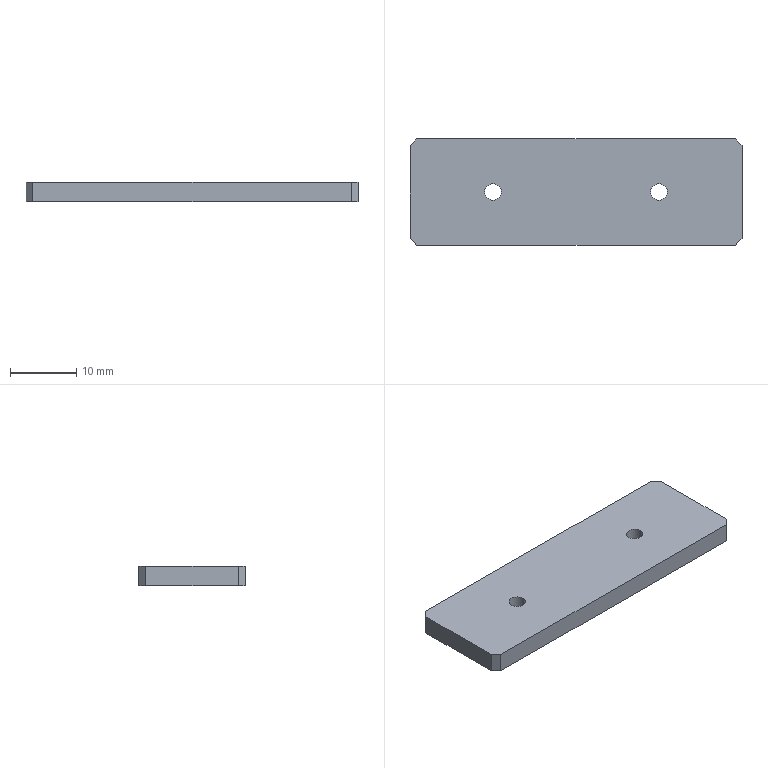Part | SolidWorks | features Chamfer 1, Extrusion 1, HoleWzd 1 | 1 solid | 14 faces | box 50 x 16 x 3 mm | volume 2365 mm3 | plane 10 | cylinder 4 | commonest cylinder face diameters 2.5 x4
STEP:
#1=CARTESIAN_POINT('',(-11.25,0.,1.5));
#2=VERTEX_POINT('',#1);
#3=CARTESIAN_POINT('',(-13.75,0.,1.5));
#4=VERTEX_POINT('',#3);
#5=CARTESIAN_POINT('',(-12.5,0.,1.5));
#6=DIRECTION('',(0.,0.,-1.));
#7=DIRECTION('',(-1.,0.,0.));
#8=AXIS2_PLACEMENT_3D('',#5,#6,#7);
#9=CIRCLE('',#8,1.25);
#10=EDGE_CURVE('',#2,#4,#9,.T.);
#11=ORIENTED_EDGE('',*,*,#10,.F.);
#12=CARTESIAN_POINT('',(-11.25,0.,-1.5));
#13=VERTEX_POINT('',#12);
#14=CARTESIAN_POINT('',(-11.25,0.,-1.5));
#15=DIRECTION('',(0.,0.,-1.));
#16=VECTOR('',#15,1000.);
#17=LINE('',#14,#16);
#18=EDGE_CURVE('',#2,#13,#17,.T.);
#19=ORIENTED_EDGE('',*,*,#18,.T.);
#20=CARTESIAN_POINT('',(-13.75,0.,-1.5));
#21=VERTEX_POINT('',#20);
#22=CARTESIAN_POINT('',(-12.5,0.,-1.5));
#23=DIRECTION('',(0.,0.,-1.));
#24=DIRECTION('',(-1.,0.,0.));
#25=AXIS2_PLACEMENT_3D('',#22,#23,#24);
#26=CIRCLE('',#25,1.25);
#27=EDGE_CURVE('',#13,#21,#26,.T.);
#28=ORIENTED_EDGE('',*,*,#27,.T.);
#29=CARTESIAN_POINT('',(-13.75,0.,-1.5));
#30=DIRECTION('',(0.,0.,-1.));
#31=VECTOR('',#30,1000.);
#32=LINE('',#29,#31);
#33=EDGE_CURVE('',#4,#21,#32,.T.);
#34=ORIENTED_EDGE('',*,*,#33,.F.);
#35=EDGE_LOOP('',(#11,#19,#28,#34));
#36=FACE_OUTER_BOUND('',#35,.T.);
#37=CARTESIAN_POINT('',(-12.5,0.,-1.5));
#38=DIRECTION('',(0.,0.,-1.));
#39=DIRECTION('',(-1.,0.,0.));
#40=AXIS2_PLACEMENT_3D('',#37,#38,#39);
#41=CYLINDRICAL_SURFACE('',#40,1.25);
#42=ADVANCED_FACE('',(#36),#41,.F.);
#43=CARTESIAN_POINT('',(13.75,0.,1.5));
#44=VERTEX_POINT('',#43);
#45=CARTESIAN_POINT('',(11.25,0.,1.5));
#46=VERTEX_POINT('',#45);
#47=CARTESIAN_POINT('',(12.5,0.,1.5));
#48=DIRECTION('',(0.,0.,-1.));
#49=DIRECTION('',(-1.,0.,0.));
#50=AXIS2_PLACEMENT_3D('',#47,#48,#49);
#51=CIRCLE('',#50,1.25);
#52=EDGE_CURVE('',#44,#46,#51,.T.);
#53=ORIENTED_EDGE('',*,*,#52,.F.);
#54=CARTESIAN_POINT('',(13.75,0.,-1.5));
#55=VERTEX_POINT('',#54);
#56=CARTESIAN_POINT('',(13.75,0.,-1.5));
#57=DIRECTION('',(0.,0.,-1.));
#58=VECTOR('',#57,1000.);
#59=LINE('',#56,#58);
#60=EDGE_CURVE('',#44,#55,#59,.T.);
#61=ORIENTED_EDGE('',*,*,#60,.T.);
#62=CARTESIAN_POINT('',(11.25,0.,-1.5));
#63=VERTEX_POINT('',#62);
#64=CARTESIAN_POINT('',(12.5,0.,-1.5));
#65=DIRECTION('',(0.,0.,-1.));
#66=DIRECTION('',(-1.,0.,0.));
#67=AXIS2_PLACEMENT_3D('',#64,#65,#66);
#68=CIRCLE('',#67,1.25);
#69=EDGE_CURVE('',#55,#63,#68,.T.);
#70=ORIENTED_EDGE('',*,*,#69,.T.);
#71=CARTESIAN_POINT('',(11.25,0.,-1.5));
#72=DIRECTION('',(0.,0.,-1.));
#73=VECTOR('',#72,1000.);
#74=LINE('',#71,#73);
#75=EDGE_CURVE('',#46,#63,#74,.T.);
#76=ORIENTED_EDGE('',*,*,#75,.F.);
#77=EDGE_LOOP('',(#53,#61,#70,#76));
#78=FACE_OUTER_BOUND('',#77,.T.);
#79=CARTESIAN_POINT('',(12.5,0.,-1.5));
#80=DIRECTION('',(0.,0.,-1.));
#81=DIRECTION('',(-1.,0.,0.));
#82=AXIS2_PLACEMENT_3D('',#79,#80,#81);
#83=CYLINDRICAL_SURFACE('',#82,1.25);
#84=ADVANCED_FACE('',(#78),#83,.F.);
#85=CARTESIAN_POINT('',(25.,-7.,1.5));
#86=VERTEX_POINT('',#85);
#87=CARTESIAN_POINT('',(25.,7.,1.5));
#88=VERTEX_POINT('',#87);
#89=CARTESIAN_POINT('',(25.,8.,1.5));
#90=DIRECTION('',(0.,1.,0.));
#91=VECTOR('',#90,1000.);
#92=LINE('',#89,#91);
#93=EDGE_CURVE('',#86,#88,#92,.T.);
#94=ORIENTED_EDGE('',*,*,#93,.F.);
#95=CARTESIAN_POINT('',(25.,-7.,-1.5));
#96=VERTEX_POINT('',#95);
#97=CARTESIAN_POINT('',(25.,-7.,1.5));
#98=DIRECTION('',(0.,0.,-1.));
#99=VECTOR('',#98,1000.);
#100=LINE('',#97,#99);
#101=EDGE_CURVE('',#86,#96,#100,.T.);
#102=ORIENTED_EDGE('',*,*,#101,.T.);
#103=CARTESIAN_POINT('',(25.,7.,-1.5));
#104=VERTEX_POINT('',#103);
#105=CARTESIAN_POINT('',(25.,8.,-1.5));
#106=DIRECTION('',(0.,1.,0.));
#107=VECTOR('',#106,1000.);
#108=LINE('',#105,#107);
#109=EDGE_CURVE('',#96,#104,#108,.T.);
#110=ORIENTED_EDGE('',*,*,#109,.T.);
#111=CARTESIAN_POINT('',(25.,7.,1.5));
#112=DIRECTION('',(0.,0.,1.));
#113=VECTOR('',#112,1000.);
#114=LINE('',#111,#113);
#115=EDGE_CURVE('',#104,#88,#114,.T.);
#116=ORIENTED_EDGE('',*,*,#115,.T.);
#117=EDGE_LOOP('',(#94,#102,#110,#116));
#118=FACE_OUTER_BOUND('',#117,.T.);
#119=CARTESIAN_POINT('',(25.,8.,1.5));
#120=DIRECTION('',(-1.,0.,0.));
#121=DIRECTION('',(0.,-1.,0.));
#122=AXIS2_PLACEMENT_3D('',#119,#120,#121);
#123=PLANE('',#122);
#124=ADVANCED_FACE('',(#118),#123,.F.);
#125=CARTESIAN_POINT('',(24.,8.,-1.5));
#126=VERTEX_POINT('',#125);
#127=CARTESIAN_POINT('',(-24.,8.,-1.5));
#128=VERTEX_POINT('',#127);
#129=CARTESIAN_POINT('',(-25.,8.,-1.5));
#130=DIRECTION('',(-1.,0.,0.));
#131=VECTOR('',#130,1000.);
#132=LINE('',#129,#131);
#133=EDGE_CURVE('',#126,#128,#132,.T.);
#134=ORIENTED_EDGE('',*,*,#133,.T.);
#135=CARTESIAN_POINT('',(-24.,8.,1.5));
#136=VERTEX_POINT('',#135);
#137=CARTESIAN_POINT('',(-24.,8.,1.5));
#138=DIRECTION('',(0.,0.,1.));
#139=VECTOR('',#138,1000.);
#140=LINE('',#137,#139);
#141=EDGE_CURVE('',#128,#136,#140,.T.);
#142=ORIENTED_EDGE('',*,*,#141,.T.);
#143=CARTESIAN_POINT('',(24.,8.,1.5));
#144=VERTEX_POINT('',#143);
#145=CARTESIAN_POINT('',(-25.,8.,1.5));
#146=DIRECTION('',(-1.,0.,0.));
#147=VECTOR('',#146,1000.);
#148=LINE('',#145,#147);
#149=EDGE_CURVE('',#144,#136,#148,.T.);
#150=ORIENTED_EDGE('',*,*,#149,.F.);
#151=CARTESIAN_POINT('',(24.,8.,1.5));
#152=DIRECTION('',(0.,0.,-1.));
#153=VECTOR('',#152,1000.);
#154=LINE('',#151,#153);
#155=EDGE_CURVE('',#144,#126,#154,.T.);
#156=ORIENTED_EDGE('',*,*,#155,.T.);
#157=EDGE_LOOP('',(#134,#142,#150,#156));
#158=FACE_OUTER_BOUND('',#157,.T.);
#159=CARTESIAN_POINT('',(-25.,8.,1.5));
#160=DIRECTION('',(0.,-1.,0.));
#161=DIRECTION('',(0.,0.,-1.));
#162=AXIS2_PLACEMENT_3D('',#159,#160,#161);
#163=PLANE('',#162);
#164=ADVANCED_FACE('',(#158),#163,.F.);
#165=CARTESIAN_POINT('',(-25.,7.,-1.5));
#166=VERTEX_POINT('',#165);
#167=CARTESIAN_POINT('',(-25.,-7.,-1.5));
#168=VERTEX_POINT('',#167);
#169=CARTESIAN_POINT('',(-25.,8.,-1.5));
#170=DIRECTION('',(0.,-1.,0.));
#171=VECTOR('',#170,1000.);
#172=LINE('',#169,#171);
#173=EDGE_CURVE('',#166,#168,#172,.T.);
#174=ORIENTED_EDGE('',*,*,#173,.T.);
#175=CARTESIAN_POINT('',(-25.,-7.,1.5));
#176=VERTEX_POINT('',#175);
#177=CARTESIAN_POINT('',(-25.,-7.,1.5));
#178=DIRECTION('',(0.,0.,1.));
#179=VECTOR('',#178,1000.);
#180=LINE('',#177,#179);
#181=EDGE_CURVE('',#168,#176,#180,.T.);
#182=ORIENTED_EDGE('',*,*,#181,.T.);
#183=CARTESIAN_POINT('',(-25.,7.,1.5));
#184=VERTEX_POINT('',#183);
#185=CARTESIAN_POINT('',(-25.,8.,1.5));
#186=DIRECTION('',(0.,-1.,0.));
#187=VECTOR('',#186,1000.);
#188=LINE('',#185,#187);
#189=EDGE_CURVE('',#184,#176,#188,.T.);
#190=ORIENTED_EDGE('',*,*,#189,.F.);
#191=CARTESIAN_POINT('',(-25.,7.,1.5));
#192=DIRECTION('',(0.,0.,-1.));
#193=VECTOR('',#192,1000.);
#194=LINE('',#191,#193);
#195=EDGE_CURVE('',#184,#166,#194,.T.);
#196=ORIENTED_EDGE('',*,*,#195,.T.);
#197=EDGE_LOOP('',(#174,#182,#190,#196));
#198=FACE_OUTER_BOUND('',#197,.T.);
#199=CARTESIAN_POINT('',(-25.,8.,1.5));
#200=DIRECTION('',(1.,0.,0.));
#201=DIRECTION('',(0.,0.,-1.));
#202=AXIS2_PLACEMENT_3D('',#199,#200,#201);
#203=PLANE('',#202);
#204=ADVANCED_FACE('',(#198),#203,.F.);
#205=CARTESIAN_POINT('',(-24.,-8.,1.5));
#206=VERTEX_POINT('',#205);
#207=CARTESIAN_POINT('',(24.,-8.,1.5));
#208=VERTEX_POINT('',#207);
#209=CARTESIAN_POINT('',(-25.,-8.,1.5));
#210=DIRECTION('',(1.,0.,0.));
#211=VECTOR('',#210,1000.);
#212=LINE('',#209,#211);
#213=EDGE_CURVE('',#206,#208,#212,.T.);
#214=ORIENTED_EDGE('',*,*,#213,.F.);
#215=CARTESIAN_POINT('',(-24.,-8.,-1.5));
#216=VERTEX_POINT('',#215);
#217=CARTESIAN_POINT('',(-24.,-8.,1.5));
#218=DIRECTION('',(0.,0.,-1.));
#219=VECTOR('',#218,1000.);
#220=LINE('',#217,#219);
#221=EDGE_CURVE('',#206,#216,#220,.T.);
#222=ORIENTED_EDGE('',*,*,#221,.T.);
#223=CARTESIAN_POINT('',(24.,-8.,-1.5));
#224=VERTEX_POINT('',#223);
#225=CARTESIAN_POINT('',(-25.,-8.,-1.5));
#226=DIRECTION('',(1.,0.,0.));
#227=VECTOR('',#226,1000.);
#228=LINE('',#225,#227);
#229=EDGE_CURVE('',#216,#224,#228,.T.);
#230=ORIENTED_EDGE('',*,*,#229,.T.);
#231=CARTESIAN_POINT('',(24.,-8.,1.5));
#232=DIRECTION('',(0.,0.,1.));
#233=VECTOR('',#232,1000.);
#234=LINE('',#231,#233);
#235=EDGE_CURVE('',#224,#208,#234,.T.);
#236=ORIENTED_EDGE('',*,*,#235,.T.);
#237=EDGE_LOOP('',(#214,#222,#230,#236));
#238=FACE_OUTER_BOUND('',#237,.T.);
#239=CARTESIAN_POINT('',(-25.,-8.,1.5));
#240=DIRECTION('',(0.,1.,0.));
#241=DIRECTION('',(0.,0.,1.));
#242=AXIS2_PLACEMENT_3D('',#239,#240,#241);
#243=PLANE('',#242);
#244=ADVANCED_FACE('',(#238),#243,.F.);
#245=CARTESIAN_POINT('',(-12.5,0.,1.5));
#246=DIRECTION('',(0.,0.,-1.));
#247=DIRECTION('',(-1.,0.,0.));
#248=AXIS2_PLACEMENT_3D('',#245,#246,#247);
#249=CIRCLE('',#248,1.25);
#250=EDGE_CURVE('',#4,#2,#249,.T.);
#251=ORIENTED_EDGE('',*,*,#250,.T.);
#252=ORIENTED_EDGE('',*,*,#10,.T.);
#253=EDGE_LOOP('',(#251,#252));
#254=FACE_BOUND('',#253,.T.);
#255=CARTESIAN_POINT('',(12.5,0.,1.5));
#256=DIRECTION('',(0.,0.,-1.));
#257=DIRECTION('',(-1.,0.,0.));
#258=AXIS2_PLACEMENT_3D('',#255,#256,#257);
#259=CIRCLE('',#258,1.25);
#260=EDGE_CURVE('',#46,#44,#259,.T.);
#261=ORIENTED_EDGE('',*,*,#260,.T.);
#262=ORIENTED_EDGE('',*,*,#52,.T.);
#263=EDGE_LOOP('',(#261,#262));
#264=FACE_BOUND('',#263,.T.);
#265=ORIENTED_EDGE('',*,*,#189,.T.);
#266=CARTESIAN_POINT('',(-16.,-16.,1.5));
#267=DIRECTION('',(0.7071,-0.7071,0.));
#268=VECTOR('',#267,1000.);
#269=LINE('',#266,#268);
#270=EDGE_CURVE('',#176,#206,#269,.T.);
#271=ORIENTED_EDGE('',*,*,#270,.T.);
#272=ORIENTED_EDGE('',*,*,#213,.T.);
#273=CARTESIAN_POINT('',(16.,-16.,1.5));
#274=DIRECTION('',(0.7071,0.7071,0.));
#275=VECTOR('',#274,1000.);
#276=LINE('',#273,#275);
#277=EDGE_CURVE('',#208,#86,#276,.T.);
#278=ORIENTED_EDGE('',*,*,#277,.T.);
#279=ORIENTED_EDGE('',*,*,#93,.T.);
#280=CARTESIAN_POINT('',(16.,16.,1.5));
#281=DIRECTION('',(-0.7071,0.7071,0.));
#282=VECTOR('',#281,1000.);
#283=LINE('',#280,#282);
#284=EDGE_CURVE('',#88,#144,#283,.T.);
#285=ORIENTED_EDGE('',*,*,#284,.T.);
#286=ORIENTED_EDGE('',*,*,#149,.T.);
#287=CARTESIAN_POINT('',(-16.,16.,1.5));
#288=DIRECTION('',(-0.7071,-0.7071,0.));
#289=VECTOR('',#288,1000.);
#290=LINE('',#287,#289);
#291=EDGE_CURVE('',#136,#184,#290,.T.);
#292=ORIENTED_EDGE('',*,*,#291,.T.);
#293=EDGE_LOOP('',(#265,#271,#272,#278,#279,#285,#286,#292));
#294=FACE_OUTER_BOUND('',#293,.T.);
#295=CARTESIAN_POINT('',(0.,0.,1.5));
#296=DIRECTION('',(0.,0.,1.));
#297=DIRECTION('',(1.,0.,0.));
#298=AXIS2_PLACEMENT_3D('',#295,#296,#297);
#299=PLANE('',#298);
#300=ADVANCED_FACE('',(#254,#264,#294),#299,.T.);
#301=CARTESIAN_POINT('',(-12.5,0.,-1.5));
#302=DIRECTION('',(0.,0.,-1.));
#303=DIRECTION('',(-1.,0.,0.));
#304=AXIS2_PLACEMENT_3D('',#301,#302,#303);
#305=CIRCLE('',#304,1.25);
#306=EDGE_CURVE('',#21,#13,#305,.T.);
#307=ORIENTED_EDGE('',*,*,#306,.F.);
#308=ORIENTED_EDGE('',*,*,#27,.F.);
#309=EDGE_LOOP('',(#307,#308));
#310=FACE_BOUND('',#309,.T.);
#311=CARTESIAN_POINT('',(12.5,0.,-1.5));
#312=DIRECTION('',(0.,0.,-1.));
#313=DIRECTION('',(-1.,0.,0.));
#314=AXIS2_PLACEMENT_3D('',#311,#312,#313);
#315=CIRCLE('',#314,1.25);
#316=EDGE_CURVE('',#63,#55,#315,.T.);
#317=ORIENTED_EDGE('',*,*,#316,.F.);
#318=ORIENTED_EDGE('',*,*,#69,.F.);
#319=EDGE_LOOP('',(#317,#318));
#320=FACE_BOUND('',#319,.T.);
#321=ORIENTED_EDGE('',*,*,#229,.F.);
#322=CARTESIAN_POINT('',(-24.,-8.,-1.5));
#323=DIRECTION('',(-0.7071,0.7071,0.));
#324=VECTOR('',#323,1000.);
#325=LINE('',#322,#324);
#326=EDGE_CURVE('',#216,#168,#325,.T.);
#327=ORIENTED_EDGE('',*,*,#326,.T.);
#328=ORIENTED_EDGE('',*,*,#173,.F.);
#329=CARTESIAN_POINT('',(-25.,7.,-1.5));
#330=DIRECTION('',(0.7071,0.7071,0.));
#331=VECTOR('',#330,1000.);
#332=LINE('',#329,#331);
#333=EDGE_CURVE('',#166,#128,#332,.T.);
#334=ORIENTED_EDGE('',*,*,#333,.T.);
#335=ORIENTED_EDGE('',*,*,#133,.F.);
#336=CARTESIAN_POINT('',(24.,8.,-1.5));
#337=DIRECTION('',(0.7071,-0.7071,0.));
#338=VECTOR('',#337,1000.);
#339=LINE('',#336,#338);
#340=EDGE_CURVE('',#126,#104,#339,.T.);
#341=ORIENTED_EDGE('',*,*,#340,.T.);
#342=ORIENTED_EDGE('',*,*,#109,.F.);
#343=CARTESIAN_POINT('',(25.,-7.,-1.5));
#344=DIRECTION('',(-0.7071,-0.7071,0.));
#345=VECTOR('',#344,1000.);
#346=LINE('',#343,#345);
#347=EDGE_CURVE('',#96,#224,#346,.T.);
#348=ORIENTED_EDGE('',*,*,#347,.T.);
#349=EDGE_LOOP('',(#321,#327,#328,#334,#335,#341,#342,#348));
#350=FACE_OUTER_BOUND('',#349,.T.);
#351=CARTESIAN_POINT('',(0.,0.,-1.5));
#352=DIRECTION('',(0.,0.,1.));
#353=DIRECTION('',(1.,0.,0.));
#354=AXIS2_PLACEMENT_3D('',#351,#352,#353);
#355=PLANE('',#354);
#356=ADVANCED_FACE('',(#310,#320,#350),#355,.F.);
#357=ORIENTED_EDGE('',*,*,#60,.F.);
#358=ORIENTED_EDGE('',*,*,#260,.F.);
#359=ORIENTED_EDGE('',*,*,#75,.T.);
#360=ORIENTED_EDGE('',*,*,#316,.T.);
#361=EDGE_LOOP('',(#357,#358,#359,#360));
#362=FACE_OUTER_BOUND('',#361,.T.);
#363=CARTESIAN_POINT('',(12.5,0.,-1.5));
#364=DIRECTION('',(0.,0.,-1.));
#365=DIRECTION('',(-1.,0.,0.));
#366=AXIS2_PLACEMENT_3D('',#363,#364,#365);
#367=CYLINDRICAL_SURFACE('',#366,1.25);
#368=ADVANCED_FACE('',(#362),#367,.F.);
#369=ORIENTED_EDGE('',*,*,#18,.F.);
#370=ORIENTED_EDGE('',*,*,#250,.F.);
#371=ORIENTED_EDGE('',*,*,#33,.T.);
#372=ORIENTED_EDGE('',*,*,#306,.T.);
#373=EDGE_LOOP('',(#369,#370,#371,#372));
#374=FACE_OUTER_BOUND('',#373,.T.);
#375=CARTESIAN_POINT('',(-12.5,0.,-1.5));
#376=DIRECTION('',(0.,0.,-1.));
#377=DIRECTION('',(-1.,0.,0.));
#378=AXIS2_PLACEMENT_3D('',#375,#376,#377);
#379=CYLINDRICAL_SURFACE('',#378,1.25);
#380=ADVANCED_FACE('',(#374),#379,.F.);
#381=ORIENTED_EDGE('',*,*,#270,.F.);
#382=ORIENTED_EDGE('',*,*,#181,.F.);
#383=ORIENTED_EDGE('',*,*,#326,.F.);
#384=ORIENTED_EDGE('',*,*,#221,.F.);
#385=EDGE_LOOP('',(#381,#382,#383,#384));
#386=FACE_OUTER_BOUND('',#385,.T.);
#387=CARTESIAN_POINT('',(-24.,-8.,1.5));
#388=DIRECTION('',(0.7071,0.7071,0.));
#389=DIRECTION('',(0.,0.,-1.));
#390=AXIS2_PLACEMENT_3D('',#387,#388,#389);
#391=PLANE('',#390);
#392=ADVANCED_FACE('',(#386),#391,.F.);
#393=ORIENTED_EDGE('',*,*,#291,.F.);
#394=ORIENTED_EDGE('',*,*,#141,.F.);
#395=ORIENTED_EDGE('',*,*,#333,.F.);
#396=ORIENTED_EDGE('',*,*,#195,.F.);
#397=EDGE_LOOP('',(#393,#394,#395,#396));
#398=FACE_OUTER_BOUND('',#397,.T.);
#399=CARTESIAN_POINT('',(-25.,7.,1.5));
#400=DIRECTION('',(0.7071,-0.7071,0.));
#401=DIRECTION('',(0.,0.,-1.));
#402=AXIS2_PLACEMENT_3D('',#399,#400,#401);
#403=PLANE('',#402);
#404=ADVANCED_FACE('',(#398),#403,.F.);
#405=ORIENTED_EDGE('',*,*,#277,.F.);
#406=ORIENTED_EDGE('',*,*,#235,.F.);
#407=ORIENTED_EDGE('',*,*,#347,.F.);
#408=ORIENTED_EDGE('',*,*,#101,.F.);
#409=EDGE_LOOP('',(#405,#406,#407,#408));
#410=FACE_OUTER_BOUND('',#409,.T.);
#411=CARTESIAN_POINT('',(25.,-7.,1.5));
#412=DIRECTION('',(-0.7071,0.7071,0.));
#413=DIRECTION('',(0.,0.,-1.));
#414=AXIS2_PLACEMENT_3D('',#411,#412,#413);
#415=PLANE('',#414);
#416=ADVANCED_FACE('',(#410),#415,.F.);
#417=ORIENTED_EDGE('',*,*,#284,.F.);
#418=ORIENTED_EDGE('',*,*,#115,.F.);
#419=ORIENTED_EDGE('',*,*,#340,.F.);
#420=ORIENTED_EDGE('',*,*,#155,.F.);
#421=EDGE_LOOP('',(#417,#418,#419,#420));
#422=FACE_OUTER_BOUND('',#421,.T.);
#423=CARTESIAN_POINT('',(24.,8.,1.5));
#424=DIRECTION('',(-0.7071,-0.7071,0.));
#425=DIRECTION('',(0.,0.,-1.));
#426=AXIS2_PLACEMENT_3D('',#423,#424,#425);
#427=PLANE('',#426);
#428=ADVANCED_FACE('',(#422),#427,.F.);
#429=CLOSED_SHELL('',(#42,#84,#124,#164,#204,#244,#300,#356,#368,#380,#392,#404,#416,#428));
#430=MANIFOLD_SOLID_BREP('',#429);
#431=CARTESIAN_POINT('',(0.,0.,0.));
#432=DIRECTION('',(0.,0.,1.));
#433=DIRECTION('',(1.,0.,0.));
#434=AXIS2_PLACEMENT_3D('',#431,#432,#433);
#435=(LENGTH_UNIT()NAMED_UNIT(*)SI_UNIT(.MILLI.,.METRE.));
#436=UNCERTAINTY_MEASURE_WITH_UNIT(LENGTH_MEASURE(0.00001),#435,'','');
#437=(NAMED_UNIT(*)PLANE_ANGLE_UNIT()SI_UNIT($,.RADIAN.));
#438=(NAMED_UNIT(*)SI_UNIT($,.STERADIAN.)SOLID_ANGLE_UNIT());
#439=(GEOMETRIC_REPRESENTATION_CONTEXT(3)GLOBAL_UNCERTAINTY_ASSIGNED_CONTEXT((#436))GLOBAL_UNIT_ASSIGNED_CONTEXT((#435,#437,#438))REPRESENTATION_CONTEXT('',''));
#440=ADVANCED_BREP_SHAPE_REPRESENTATION('',(#430,#434),#439);